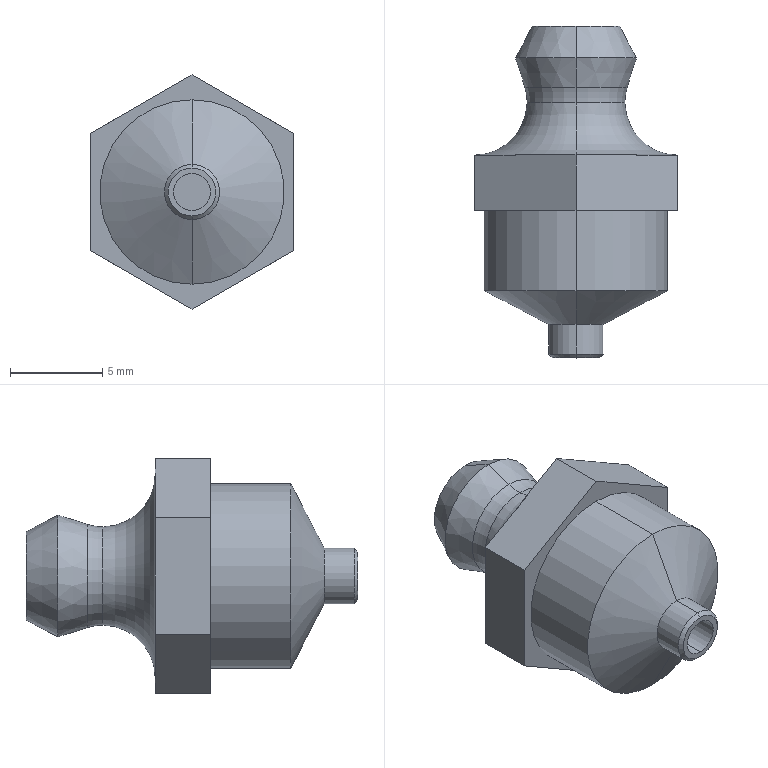Part | SolidWorks | features Boss 1, Chamfer 1, Revolution 1 | 1 solid | 37 faces | box 11 x 18 x 12.702 mm | volume 898.201 mm3 | plane 17 | cone 8 | cylinder 8 | torus 4 | commonest cylinder face diameters 2 x4 3 x2 10 x2
STEP:
#1=CARTESIAN_POINT('',(0.,14.676,2.8));
#2=VERTEX_POINT('',#1);
#3=CARTESIAN_POINT('',(0.,13.829,2.671));
#4=VERTEX_POINT('',#3);
#5=CARTESIAN_POINT('',(0.,13.829,5.5));
#6=DIRECTION('',(-1.,0.,0.));
#7=DIRECTION('',(0.,0.,1.));
#8=AXIS2_PLACEMENT_3D('',#5,#6,#7);
#9=CIRCLE('',#8,2.829);
#10=EDGE_CURVE('',#2,#4,#9,.T.);
#11=ORIENTED_EDGE('',*,*,#10,.T.);
#12=CARTESIAN_POINT('',(0.,13.829,-2.671));
#13=VERTEX_POINT('',#12);
#14=CARTESIAN_POINT('',(0.,13.829,0.));
#15=DIRECTION('',(0.,1.,0.));
#16=DIRECTION('',(0.,0.,1.));
#17=AXIS2_PLACEMENT_3D('',#14,#15,#16);
#18=CIRCLE('',#17,2.671);
#19=EDGE_CURVE('',#4,#13,#18,.T.);
#20=ORIENTED_EDGE('',*,*,#19,.T.);
#21=CARTESIAN_POINT('',(0.,14.676,-2.8));
#22=VERTEX_POINT('',#21);
#23=CARTESIAN_POINT('',(0.,13.829,-5.5));
#24=DIRECTION('',(1.,0.,0.));
#25=DIRECTION('',(0.,0.,-1.));
#26=AXIS2_PLACEMENT_3D('',#23,#24,#25);
#27=CIRCLE('',#26,2.829);
#28=EDGE_CURVE('',#22,#13,#27,.T.);
#29=ORIENTED_EDGE('',*,*,#28,.F.);
#30=CARTESIAN_POINT('',(0.,14.676,0.));
#31=DIRECTION('',(0.,1.,0.));
#32=DIRECTION('',(0.,0.,1.));
#33=AXIS2_PLACEMENT_3D('',#30,#31,#32);
#34=CIRCLE('',#33,2.8);
#35=EDGE_CURVE('',#2,#22,#34,.T.);
#36=ORIENTED_EDGE('',*,*,#35,.F.);
#37=EDGE_LOOP('',(#11,#20,#29,#36));
#38=FACE_OUTER_BOUND('',#37,.T.);
#39=CARTESIAN_POINT('',(0.,13.829,0.));
#40=DIRECTION('',(0.,1.,0.));
#41=DIRECTION('',(0.,0.,1.));
#42=AXIS2_PLACEMENT_3D('',#39,#40,#41);
#43=TOROIDAL_SURFACE('',#42,5.5,2.829);
#44=ADVANCED_FACE('',(#38),#43,.F.);
#45=ORIENTED_EDGE('',*,*,#28,.T.);
#46=CARTESIAN_POINT('',(0.,13.829,0.));
#47=DIRECTION('',(0.,1.,0.));
#48=DIRECTION('',(0.,0.,1.));
#49=AXIS2_PLACEMENT_3D('',#46,#47,#48);
#50=CIRCLE('',#49,2.671);
#51=EDGE_CURVE('',#13,#4,#50,.T.);
#52=ORIENTED_EDGE('',*,*,#51,.T.);
#53=ORIENTED_EDGE('',*,*,#10,.F.);
#54=CARTESIAN_POINT('',(0.,14.676,0.));
#55=DIRECTION('',(0.,1.,0.));
#56=DIRECTION('',(0.,0.,1.));
#57=AXIS2_PLACEMENT_3D('',#54,#55,#56);
#58=CIRCLE('',#57,2.8);
#59=EDGE_CURVE('',#22,#2,#58,.T.);
#60=ORIENTED_EDGE('',*,*,#59,.F.);
#61=EDGE_LOOP('',(#45,#52,#53,#60));
#62=FACE_OUTER_BOUND('',#61,.T.);
#63=CARTESIAN_POINT('',(0.,13.829,0.));
#64=DIRECTION('',(0.,1.,0.));
#65=DIRECTION('',(0.,0.,1.));
#66=AXIS2_PLACEMENT_3D('',#63,#64,#65);
#67=TOROIDAL_SURFACE('',#66,5.5,2.829);
#68=ADVANCED_FACE('',(#62),#67,.F.);
#69=CARTESIAN_POINT('',(0.,0.,-1.3));
#70=VERTEX_POINT('',#69);
#71=CARTESIAN_POINT('',(0.,0.,1.3));
#72=VERTEX_POINT('',#71);
#73=CARTESIAN_POINT('',(0.,0.,0.));
#74=DIRECTION('',(0.,-1.,0.));
#75=DIRECTION('',(0.,0.,-1.));
#76=AXIS2_PLACEMENT_3D('',#73,#74,#75);
#77=CIRCLE('',#76,1.3);
#78=EDGE_CURVE('',#70,#72,#77,.T.);
#79=ORIENTED_EDGE('',*,*,#78,.F.);
#80=CARTESIAN_POINT('',(0.,0.2,-1.5));
#81=VERTEX_POINT('',#80);
#82=CARTESIAN_POINT('',(0.,0.2,-1.5));
#83=DIRECTION('',(0.,0.7071,-0.7071));
#84=VECTOR('',#83,1000.);
#85=LINE('',#82,#84);
#86=EDGE_CURVE('',#70,#81,#85,.T.);
#87=ORIENTED_EDGE('',*,*,#86,.T.);
#88=CARTESIAN_POINT('',(0.,0.2,1.5));
#89=VERTEX_POINT('',#88);
#90=CARTESIAN_POINT('',(0.,0.2,0.));
#91=DIRECTION('',(0.,1.,0.));
#92=DIRECTION('',(0.,0.,-1.));
#93=AXIS2_PLACEMENT_3D('',#90,#91,#92);
#94=CIRCLE('',#93,1.5);
#95=EDGE_CURVE('',#89,#81,#94,.T.);
#96=ORIENTED_EDGE('',*,*,#95,.F.);
#97=CARTESIAN_POINT('',(0.,0.2,1.5));
#98=DIRECTION('',(0.,0.7071,0.7071));
#99=VECTOR('',#98,1000.);
#100=LINE('',#97,#99);
#101=EDGE_CURVE('',#72,#89,#100,.T.);
#102=ORIENTED_EDGE('',*,*,#101,.F.);
#103=EDGE_LOOP('',(#79,#87,#96,#102));
#104=FACE_OUTER_BOUND('',#103,.T.);
#105=CARTESIAN_POINT('',(0.,0.2,0.));
#106=DIRECTION('',(0.,1.,0.));
#107=DIRECTION('',(0.,0.,1.));
#108=AXIS2_PLACEMENT_3D('',#105,#106,#107);
#109=CONICAL_SURFACE('',#108,1.5,0.7854);
#110=ADVANCED_FACE('',(#104),#109,.T.);
#111=ORIENTED_EDGE('',*,*,#51,.F.);
#112=CARTESIAN_POINT('',(0.,11.,-5.5));
#113=VERTEX_POINT('',#112);
#114=CARTESIAN_POINT('',(0.,13.829,-5.5));
#115=DIRECTION('',(1.,0.,0.));
#116=DIRECTION('',(0.,0.,-1.));
#117=AXIS2_PLACEMENT_3D('',#114,#115,#116);
#118=CIRCLE('',#117,2.829);
#119=EDGE_CURVE('',#13,#113,#118,.T.);
#120=ORIENTED_EDGE('',*,*,#119,.T.);
#121=CARTESIAN_POINT('',(-2.75,11.,-4.763));
#122=VERTEX_POINT('',#121);
#123=CARTESIAN_POINT('',(0.,11.,0.));
#124=DIRECTION('',(0.,1.,0.));
#125=DIRECTION('',(0.,0.,1.));
#126=AXIS2_PLACEMENT_3D('',#123,#124,#125);
#127=CIRCLE('',#126,5.5);
#128=EDGE_CURVE('',#113,#122,#127,.T.);
#129=ORIENTED_EDGE('',*,*,#128,.T.);
#130=CARTESIAN_POINT('',(-5.5,11.,0.));
#131=VERTEX_POINT('',#130);
#132=CARTESIAN_POINT('',(0.,11.,0.));
#133=DIRECTION('',(0.,1.,0.));
#134=DIRECTION('',(0.,0.,1.));
#135=AXIS2_PLACEMENT_3D('',#132,#133,#134);
#136=CIRCLE('',#135,5.5);
#137=EDGE_CURVE('',#122,#131,#136,.T.);
#138=ORIENTED_EDGE('',*,*,#137,.T.);
#139=CARTESIAN_POINT('',(-2.75,11.,4.763));
#140=VERTEX_POINT('',#139);
#141=CARTESIAN_POINT('',(0.,11.,0.));
#142=DIRECTION('',(0.,1.,0.));
#143=DIRECTION('',(0.,0.,1.));
#144=AXIS2_PLACEMENT_3D('',#141,#142,#143);
#145=CIRCLE('',#144,5.5);
#146=EDGE_CURVE('',#131,#140,#145,.T.);
#147=ORIENTED_EDGE('',*,*,#146,.T.);
#148=CARTESIAN_POINT('',(0.,11.,5.5));
#149=VERTEX_POINT('',#148);
#150=CARTESIAN_POINT('',(0.,11.,0.));
#151=DIRECTION('',(0.,1.,0.));
#152=DIRECTION('',(0.,0.,1.));
#153=AXIS2_PLACEMENT_3D('',#150,#151,#152);
#154=CIRCLE('',#153,5.5);
#155=EDGE_CURVE('',#140,#149,#154,.T.);
#156=ORIENTED_EDGE('',*,*,#155,.T.);
#157=CARTESIAN_POINT('',(0.,13.829,5.5));
#158=DIRECTION('',(-1.,0.,0.));
#159=DIRECTION('',(0.,0.,1.));
#160=AXIS2_PLACEMENT_3D('',#157,#158,#159);
#161=CIRCLE('',#160,2.829);
#162=EDGE_CURVE('',#4,#149,#161,.T.);
#163=ORIENTED_EDGE('',*,*,#162,.F.);
#164=EDGE_LOOP('',(#111,#120,#129,#138,#147,#156,#163));
#165=FACE_OUTER_BOUND('',#164,.T.);
#166=CARTESIAN_POINT('',(0.,13.829,0.));
#167=DIRECTION('',(0.,1.,0.));
#168=DIRECTION('',(0.,0.,1.));
#169=AXIS2_PLACEMENT_3D('',#166,#167,#168);
#170=TOROIDAL_SURFACE('',#169,5.5,2.829);
#171=ADVANCED_FACE('',(#165),#170,.F.);
#172=ORIENTED_EDGE('',*,*,#35,.T.);
#173=CARTESIAN_POINT('',(0.,16.271,-3.3));
#174=VERTEX_POINT('',#173);
#175=CARTESIAN_POINT('',(0.,16.271,-3.3));
#176=DIRECTION('',(0.,0.9542,-0.299));
#177=VECTOR('',#176,1000.);
#178=LINE('',#175,#177);
#179=EDGE_CURVE('',#22,#174,#178,.T.);
#180=ORIENTED_EDGE('',*,*,#179,.T.);
#181=CARTESIAN_POINT('',(0.,16.271,3.3));
#182=VERTEX_POINT('',#181);
#183=CARTESIAN_POINT('',(0.,16.271,0.));
#184=DIRECTION('',(0.,1.,0.));
#185=DIRECTION('',(0.,0.,1.));
#186=AXIS2_PLACEMENT_3D('',#183,#184,#185);
#187=CIRCLE('',#186,3.3);
#188=EDGE_CURVE('',#182,#174,#187,.T.);
#189=ORIENTED_EDGE('',*,*,#188,.F.);
#190=CARTESIAN_POINT('',(0.,16.271,3.3));
#191=DIRECTION('',(0.,0.9542,0.299));
#192=VECTOR('',#191,1000.);
#193=LINE('',#190,#192);
#194=EDGE_CURVE('',#2,#182,#193,.T.);
#195=ORIENTED_EDGE('',*,*,#194,.F.);
#196=EDGE_LOOP('',(#172,#180,#189,#195));
#197=FACE_OUTER_BOUND('',#196,.T.);
#198=CARTESIAN_POINT('',(0.,16.271,0.));
#199=DIRECTION('',(0.,1.,0.));
#200=DIRECTION('',(0.,0.,1.));
#201=AXIS2_PLACEMENT_3D('',#198,#199,#200);
#202=CONICAL_SURFACE('',#201,3.3,0.3037);
#203=ADVANCED_FACE('',(#197),#202,.T.);
#204=CARTESIAN_POINT('',(0.,18.,2.4));
#205=VERTEX_POINT('',#204);
#206=CARTESIAN_POINT('',(0.,18.,-2.4));
#207=VERTEX_POINT('',#206);
#208=CARTESIAN_POINT('',(0.,18.,0.));
#209=DIRECTION('',(0.,1.,0.));
#210=DIRECTION('',(0.,0.,1.));
#211=AXIS2_PLACEMENT_3D('',#208,#209,#210);
#212=CIRCLE('',#211,2.4);
#213=EDGE_CURVE('',#205,#207,#212,.T.);
#214=ORIENTED_EDGE('',*,*,#213,.F.);
#215=CARTESIAN_POINT('',(0.,18.,2.4));
#216=DIRECTION('',(0.,-0.887,0.4617));
#217=VECTOR('',#216,1000.);
#218=LINE('',#215,#217);
#219=EDGE_CURVE('',#205,#182,#218,.T.);
#220=ORIENTED_EDGE('',*,*,#219,.T.);
#221=ORIENTED_EDGE('',*,*,#188,.T.);
#222=CARTESIAN_POINT('',(0.,18.,-2.4));
#223=DIRECTION('',(0.,-0.887,-0.4617));
#224=VECTOR('',#223,1000.);
#225=LINE('',#222,#224);
#226=EDGE_CURVE('',#207,#174,#225,.T.);
#227=ORIENTED_EDGE('',*,*,#226,.F.);
#228=EDGE_LOOP('',(#214,#220,#221,#227));
#229=FACE_OUTER_BOUND('',#228,.T.);
#230=CARTESIAN_POINT('',(0.,18.,0.));
#231=DIRECTION('',(0.,-1.,0.));
#232=DIRECTION('',(0.,0.,-1.));
#233=AXIS2_PLACEMENT_3D('',#230,#231,#232);
#234=CONICAL_SURFACE('',#233,2.4,0.48);
#235=ADVANCED_FACE('',(#229),#234,.T.);
#236=CARTESIAN_POINT('',(0.,11.,-1.));
#237=VERTEX_POINT('',#236);
#238=CARTESIAN_POINT('',(0.,11.,1.));
#239=VERTEX_POINT('',#238);
#240=CARTESIAN_POINT('',(0.,11.,0.));
#241=DIRECTION('',(0.,1.,0.));
#242=DIRECTION('',(0.,0.,1.));
#243=AXIS2_PLACEMENT_3D('',#240,#241,#242);
#244=CIRCLE('',#243,1.);
#245=EDGE_CURVE('',#237,#239,#244,.T.);
#246=ORIENTED_EDGE('',*,*,#245,.F.);
#247=CARTESIAN_POINT('',(0.,18.,-1.));
#248=VERTEX_POINT('',#247);
#249=CARTESIAN_POINT('',(0.,0.,-1.));
#250=DIRECTION('',(0.,1.,0.));
#251=VECTOR('',#250,1000.);
#252=LINE('',#249,#251);
#253=EDGE_CURVE('',#237,#248,#252,.T.);
#254=ORIENTED_EDGE('',*,*,#253,.T.);
#255=CARTESIAN_POINT('',(0.,18.,1.));
#256=VERTEX_POINT('',#255);
#257=CARTESIAN_POINT('',(0.,18.,0.));
#258=DIRECTION('',(0.,1.,0.));
#259=DIRECTION('',(0.,0.,1.));
#260=AXIS2_PLACEMENT_3D('',#257,#258,#259);
#261=CIRCLE('',#260,1.);
#262=EDGE_CURVE('',#248,#256,#261,.T.);
#263=ORIENTED_EDGE('',*,*,#262,.T.);
#264=CARTESIAN_POINT('',(0.,0.,1.));
#265=DIRECTION('',(0.,1.,0.));
#266=VECTOR('',#265,1000.);
#267=LINE('',#264,#266);
#268=EDGE_CURVE('',#239,#256,#267,.T.);
#269=ORIENTED_EDGE('',*,*,#268,.F.);
#270=EDGE_LOOP('',(#246,#254,#263,#269));
#271=FACE_OUTER_BOUND('',#270,.T.);
#272=CARTESIAN_POINT('',(0.,0.,0.));
#273=DIRECTION('',(0.,1.,0.));
#274=DIRECTION('',(0.,0.,1.));
#275=AXIS2_PLACEMENT_3D('',#272,#273,#274);
#276=CYLINDRICAL_SURFACE('',#275,1.);
#277=ADVANCED_FACE('',(#271),#276,.F.);
#278=ORIENTED_EDGE('',*,*,#95,.T.);
#279=CARTESIAN_POINT('',(0.,1.822,-1.5));
#280=VERTEX_POINT('',#279);
#281=CARTESIAN_POINT('',(0.,0.,-1.5));
#282=DIRECTION('',(0.,1.,0.));
#283=VECTOR('',#282,1000.);
#284=LINE('',#281,#283);
#285=EDGE_CURVE('',#81,#280,#284,.T.);
#286=ORIENTED_EDGE('',*,*,#285,.T.);
#287=CARTESIAN_POINT('',(0.,1.822,1.5));
#288=VERTEX_POINT('',#287);
#289=CARTESIAN_POINT('',(0.,1.822,0.));
#290=DIRECTION('',(0.,1.,0.));
#291=DIRECTION('',(0.,0.,1.));
#292=AXIS2_PLACEMENT_3D('',#289,#290,#291);
#293=CIRCLE('',#292,1.5);
#294=EDGE_CURVE('',#288,#280,#293,.T.);
#295=ORIENTED_EDGE('',*,*,#294,.F.);
#296=CARTESIAN_POINT('',(0.,0.,1.5));
#297=DIRECTION('',(0.,1.,0.));
#298=VECTOR('',#297,1000.);
#299=LINE('',#296,#298);
#300=EDGE_CURVE('',#89,#288,#299,.T.);
#301=ORIENTED_EDGE('',*,*,#300,.F.);
#302=EDGE_LOOP('',(#278,#286,#295,#301));
#303=FACE_OUTER_BOUND('',#302,.T.);
#304=CARTESIAN_POINT('',(0.,0.,0.));
#305=DIRECTION('',(0.,1.,0.));
#306=DIRECTION('',(0.,0.,1.));
#307=AXIS2_PLACEMENT_3D('',#304,#305,#306);
#308=CYLINDRICAL_SURFACE('',#307,1.5);
#309=ADVANCED_FACE('',(#303),#308,.T.);
#310=ORIENTED_EDGE('',*,*,#294,.T.);
#311=CARTESIAN_POINT('',(0.,3.644,-5.));
#312=VERTEX_POINT('',#311);
#313=CARTESIAN_POINT('',(0.,3.644,-5.));
#314=DIRECTION('',(0.,0.4617,-0.887));
#315=VECTOR('',#314,1000.);
#316=LINE('',#313,#315);
#317=EDGE_CURVE('',#280,#312,#316,.T.);
#318=ORIENTED_EDGE('',*,*,#317,.T.);
#319=CARTESIAN_POINT('',(0.,3.644,5.));
#320=VERTEX_POINT('',#319);
#321=CARTESIAN_POINT('',(0.,3.644,0.));
#322=DIRECTION('',(0.,1.,0.));
#323=DIRECTION('',(0.,0.,1.));
#324=AXIS2_PLACEMENT_3D('',#321,#322,#323);
#325=CIRCLE('',#324,5.);
#326=EDGE_CURVE('',#320,#312,#325,.T.);
#327=ORIENTED_EDGE('',*,*,#326,.F.);
#328=CARTESIAN_POINT('',(0.,3.644,5.));
#329=DIRECTION('',(0.,0.4617,0.887));
#330=VECTOR('',#329,1000.);
#331=LINE('',#328,#330);
#332=EDGE_CURVE('',#288,#320,#331,.T.);
#333=ORIENTED_EDGE('',*,*,#332,.F.);
#334=EDGE_LOOP('',(#310,#318,#327,#333));
#335=FACE_OUTER_BOUND('',#334,.T.);
#336=CARTESIAN_POINT('',(0.,3.644,0.));
#337=DIRECTION('',(0.,1.,0.));
#338=DIRECTION('',(0.,0.,1.));
#339=AXIS2_PLACEMENT_3D('',#336,#337,#338);
#340=CONICAL_SURFACE('',#339,5.,1.091);
#341=ADVANCED_FACE('',(#335),#340,.T.);
#342=ORIENTED_EDGE('',*,*,#326,.T.);
#343=CARTESIAN_POINT('',(0.,8.,-5.));
#344=VERTEX_POINT('',#343);
#345=CARTESIAN_POINT('',(0.,0.,-5.));
#346=DIRECTION('',(0.,1.,0.));
#347=VECTOR('',#346,1000.);
#348=LINE('',#345,#347);
#349=EDGE_CURVE('',#312,#344,#348,.T.);
#350=ORIENTED_EDGE('',*,*,#349,.T.);
#351=CARTESIAN_POINT('',(0.,8.,5.));
#352=VERTEX_POINT('',#351);
#353=CARTESIAN_POINT('',(0.,8.,0.));
#354=DIRECTION('',(0.,1.,0.));
#355=DIRECTION('',(0.,0.,1.));
#356=AXIS2_PLACEMENT_3D('',#353,#354,#355);
#357=CIRCLE('',#356,5.);
#358=EDGE_CURVE('',#352,#344,#357,.T.);
#359=ORIENTED_EDGE('',*,*,#358,.F.);
#360=CARTESIAN_POINT('',(0.,0.,5.));
#361=DIRECTION('',(0.,1.,0.));
#362=VECTOR('',#361,1000.);
#363=LINE('',#360,#362);
#364=EDGE_CURVE('',#320,#352,#363,.T.);
#365=ORIENTED_EDGE('',*,*,#364,.F.);
#366=EDGE_LOOP('',(#342,#350,#359,#365));
#367=FACE_OUTER_BOUND('',#366,.T.);
#368=CARTESIAN_POINT('',(0.,0.,0.));
#369=DIRECTION('',(0.,1.,0.));
#370=DIRECTION('',(0.,0.,1.));
#371=AXIS2_PLACEMENT_3D('',#368,#369,#370);
#372=CYLINDRICAL_SURFACE('',#371,5.);
#373=ADVANCED_FACE('',(#367),#372,.T.);
#374=CARTESIAN_POINT('',(0.,0.,-1.));
#375=VERTEX_POINT('',#374);
#376=CARTESIAN_POINT('',(0.,0.,1.));
#377=VERTEX_POINT('',#376);
#378=CARTESIAN_POINT('',(0.,0.,0.));
#379=DIRECTION('',(0.,1.,0.));
#380=DIRECTION('',(0.,0.,1.));
#381=AXIS2_PLACEMENT_3D('',#378,#379,#380);
#382=CIRCLE('',#381,1.);
#383=EDGE_CURVE('',#375,#377,#382,.T.);
#384=ORIENTED_EDGE('',*,*,#383,.F.);
#385=CARTESIAN_POINT('',(0.,8.,-1.));
#386=VERTEX_POINT('',#385);
#387=CARTESIAN_POINT('',(0.,0.,-1.));
#388=DIRECTION('',(0.,1.,0.));
#389=VECTOR('',#388,1000.);
#390=LINE('',#387,#389);
#391=EDGE_CURVE('',#375,#386,#390,.T.);
#392=ORIENTED_EDGE('',*,*,#391,.T.);
#393=CARTESIAN_POINT('',(0.,8.,1.));
#394=VERTEX_POINT('',#393);
#395=CARTESIAN_POINT('',(0.,8.,0.));
#396=DIRECTION('',(0.,1.,0.));
#397=DIRECTION('',(0.,0.,1.));
#398=AXIS2_PLACEMENT_3D('',#395,#396,#397);
#399=CIRCLE('',#398,1.);
#400=EDGE_CURVE('',#386,#394,#399,.T.);
#401=ORIENTED_EDGE('',*,*,#400,.T.);
#402=CARTESIAN_POINT('',(0.,0.,1.));
#403=DIRECTION('',(0.,1.,0.));
#404=VECTOR('',#403,1000.);
#405=LINE('',#402,#404);
#406=EDGE_CURVE('',#377,#394,#405,.T.);
#407=ORIENTED_EDGE('',*,*,#406,.F.);
#408=EDGE_LOOP('',(#384,#392,#401,#407));
#409=FACE_OUTER_BOUND('',#408,.T.);
#410=CARTESIAN_POINT('',(0.,0.,0.));
#411=DIRECTION('',(0.,1.,0.));
#412=DIRECTION('',(0.,0.,1.));
#413=AXIS2_PLACEMENT_3D('',#410,#411,#412);
#414=CYLINDRICAL_SURFACE('',#413,1.);
#415=ADVANCED_FACE('',(#409),#414,.F.);
#416=ORIENTED_EDGE('',*,*,#391,.F.);
#417=CARTESIAN_POINT('',(0.,0.,0.));
#418=DIRECTION('',(0.,1.,0.));
#419=DIRECTION('',(0.,0.,1.));
#420=AXIS2_PLACEMENT_3D('',#417,#418,#419);
#421=CIRCLE('',#420,1.);
#422=EDGE_CURVE('',#377,#375,#421,.T.);
#423=ORIENTED_EDGE('',*,*,#422,.F.);
#424=ORIENTED_EDGE('',*,*,#406,.T.);
#425=CARTESIAN_POINT('',(0.,8.,0.));
#426=DIRECTION('',(0.,1.,0.));
#427=DIRECTION('',(0.,0.,1.));
#428=AXIS2_PLACEMENT_3D('',#425,#426,#427);
#429=CIRCLE('',#428,1.);
#430=EDGE_CURVE('',#394,#386,#429,.T.);
#431=ORIENTED_EDGE('',*,*,#430,.T.);
#432=EDGE_LOOP('',(#416,#423,#424,#431));
#433=FACE_OUTER_BOUND('',#432,.T.);
#434=CARTESIAN_POINT('',(0.,0.,0.));
#435=DIRECTION('',(0.,1.,0.));
#436=DIRECTION('',(0.,0.,1.));
#437=AXIS2_PLACEMENT_3D('',#434,#435,#436);
#438=CYLINDRICAL_SURFACE('',#437,1.);
#439=ADVANCED_FACE('',(#433),#438,.F.);
#440=ORIENTED_EDGE('',*,*,#358,.T.);
#441=CARTESIAN_POINT('',(0.,8.,0.));
#442=DIRECTION('',(0.,1.,0.));
#443=DIRECTION('',(0.,0.,1.));
#444=AXIS2_PLACEMENT_3D('',#441,#442,#443);
#445=CIRCLE('',#444,5.);
#446=EDGE_CURVE('',#344,#352,#445,.T.);
#447=ORIENTED_EDGE('',*,*,#446,.T.);
#448=EDGE_LOOP('',(#440,#447));
#449=FACE_BOUND('',#448,.T.);
#450=CARTESIAN_POINT('',(5.5,8.,3.175));
#451=VERTEX_POINT('',#450);
#452=CARTESIAN_POINT('',(0.,8.,6.351));
#453=VERTEX_POINT('',#452);
#454=CARTESIAN_POINT('',(5.5,8.,3.175));
#455=DIRECTION('',(-0.866,0.,0.5));
#456=VECTOR('',#455,1000.);
#457=LINE('',#454,#456);
#458=EDGE_CURVE('',#451,#453,#457,.T.);
#459=ORIENTED_EDGE('',*,*,#458,.T.);
#460=CARTESIAN_POINT('',(-5.5,8.,3.175));
#461=VERTEX_POINT('',#460);
#462=CARTESIAN_POINT('',(0.,8.,6.351));
#463=DIRECTION('',(-0.866,0.,-0.5));
#464=VECTOR('',#463,1000.);
#465=LINE('',#462,#464);
#466=EDGE_CURVE('',#453,#461,#465,.T.);
#467=ORIENTED_EDGE('',*,*,#466,.T.);
#468=CARTESIAN_POINT('',(-5.5,8.,-3.175));
#469=VERTEX_POINT('',#468);
#470=CARTESIAN_POINT('',(-5.5,8.,3.175));
#471=DIRECTION('',(0.,0.,-1.));
#472=VECTOR('',#471,1000.);
#473=LINE('',#470,#472);
#474=EDGE_CURVE('',#461,#469,#473,.T.);
#475=ORIENTED_EDGE('',*,*,#474,.T.);
#476=CARTESIAN_POINT('',(0.,8.,-6.351));
#477=VERTEX_POINT('',#476);
#478=CARTESIAN_POINT('',(-5.5,8.,-3.175));
#479=DIRECTION('',(0.866,0.,-0.5));
#480=VECTOR('',#479,1000.);
#481=LINE('',#478,#480);
#482=EDGE_CURVE('',#469,#477,#481,.T.);
#483=ORIENTED_EDGE('',*,*,#482,.T.);
#484=CARTESIAN_POINT('',(5.5,8.,-3.175));
#485=VERTEX_POINT('',#484);
#486=CARTESIAN_POINT('',(0.,8.,-6.351));
#487=DIRECTION('',(0.866,0.,0.5));
#488=VECTOR('',#487,1000.);
#489=LINE('',#486,#488);
#490=EDGE_CURVE('',#477,#485,#489,.T.);
#491=ORIENTED_EDGE('',*,*,#490,.T.);
#492=CARTESIAN_POINT('',(5.5,8.,-3.175));
#493=DIRECTION('',(0.,0.,1.));
#494=VECTOR('',#493,1000.);
#495=LINE('',#492,#494);
#496=EDGE_CURVE('',#485,#451,#495,.T.);
#497=ORIENTED_EDGE('',*,*,#496,.T.);
#498=EDGE_LOOP('',(#459,#467,#475,#483,#491,#497));
#499=FACE_OUTER_BOUND('',#498,.T.);
#500=CARTESIAN_POINT('',(-5.,8.,0.));
#501=DIRECTION('',(0.,-1.,0.));
#502=DIRECTION('',(0.,0.,-1.));
#503=AXIS2_PLACEMENT_3D('',#500,#501,#502);
#504=PLANE('',#503);
#505=ADVANCED_FACE('',(#449,#499),#504,.T.);
#506=ORIENTED_EDGE('',*,*,#349,.F.);
#507=CARTESIAN_POINT('',(0.,3.644,0.));
#508=DIRECTION('',(0.,1.,0.));
#509=DIRECTION('',(0.,0.,1.));
#510=AXIS2_PLACEMENT_3D('',#507,#508,#509);
#511=CIRCLE('',#510,5.);
#512=EDGE_CURVE('',#312,#320,#511,.T.);
#513=ORIENTED_EDGE('',*,*,#512,.T.);
#514=ORIENTED_EDGE('',*,*,#364,.T.);
#515=ORIENTED_EDGE('',*,*,#446,.F.);
#516=EDGE_LOOP('',(#506,#513,#514,#515));
#517=FACE_OUTER_BOUND('',#516,.T.);
#518=CARTESIAN_POINT('',(0.,0.,0.));
#519=DIRECTION('',(0.,1.,0.));
#520=DIRECTION('',(0.,0.,1.));
#521=AXIS2_PLACEMENT_3D('',#518,#519,#520);
#522=CYLINDRICAL_SURFACE('',#521,5.);
#523=ADVANCED_FACE('',(#517),#522,.T.);
#524=ORIENTED_EDGE('',*,*,#317,.F.);
#525=CARTESIAN_POINT('',(0.,1.822,0.));
#526=DIRECTION('',(0.,1.,0.));
#527=DIRECTION('',(0.,0.,1.));
#528=AXIS2_PLACEMENT_3D('',#525,#526,#527);
#529=CIRCLE('',#528,1.5);
#530=EDGE_CURVE('',#280,#288,#529,.T.);
#531=ORIENTED_EDGE('',*,*,#530,.T.);
#532=ORIENTED_EDGE('',*,*,#332,.T.);
#533=ORIENTED_EDGE('',*,*,#512,.F.);
#534=EDGE_LOOP('',(#524,#531,#532,#533));
#535=FACE_OUTER_BOUND('',#534,.T.);
#536=CARTESIAN_POINT('',(0.,3.644,0.));
#537=DIRECTION('',(0.,1.,0.));
#538=DIRECTION('',(0.,0.,1.));
#539=AXIS2_PLACEMENT_3D('',#536,#537,#538);
#540=CONICAL_SURFACE('',#539,5.,1.091);
#541=ADVANCED_FACE('',(#535),#540,.T.);
#542=ORIENTED_EDGE('',*,*,#285,.F.);
#543=CARTESIAN_POINT('',(0.,0.2,0.));
#544=DIRECTION('',(0.,1.,0.));
#545=DIRECTION('',(0.,0.,-1.));
#546=AXIS2_PLACEMENT_3D('',#543,#544,#545);
#547=CIRCLE('',#546,1.5);
#548=EDGE_CURVE('',#81,#89,#547,.T.);
#549=ORIENTED_EDGE('',*,*,#548,.T.);
#550=ORIENTED_EDGE('',*,*,#300,.T.);
#551=ORIENTED_EDGE('',*,*,#530,.F.);
#552=EDGE_LOOP('',(#542,#549,#550,#551));
#553=FACE_OUTER_BOUND('',#552,.T.);
#554=CARTESIAN_POINT('',(0.,0.,0.));
#555=DIRECTION('',(0.,1.,0.));
#556=DIRECTION('',(0.,0.,1.));
#557=AXIS2_PLACEMENT_3D('',#554,#555,#556);
#558=CYLINDRICAL_SURFACE('',#557,1.5);
#559=ADVANCED_FACE('',(#553),#558,.T.);
#560=CARTESIAN_POINT('',(0.,0.,0.));
#561=DIRECTION('',(0.,-1.,0.));
#562=DIRECTION('',(0.,0.,-1.));
#563=AXIS2_PLACEMENT_3D('',#560,#561,#562);
#564=CIRCLE('',#563,1.3);
#565=EDGE_CURVE('',#72,#70,#564,.T.);
#566=ORIENTED_EDGE('',*,*,#565,.T.);
#567=ORIENTED_EDGE('',*,*,#78,.T.);
#568=EDGE_LOOP('',(#566,#567));
#569=FACE_OUTER_BOUND('',#568,.T.);
#570=ORIENTED_EDGE('',*,*,#422,.T.);
#571=ORIENTED_EDGE('',*,*,#383,.T.);
#572=EDGE_LOOP('',(#570,#571));
#573=FACE_BOUND('',#572,.T.);
#574=CARTESIAN_POINT('',(-1.,0.,0.));
#575=DIRECTION('',(0.,-1.,0.));
#576=DIRECTION('',(0.,0.,-1.));
#577=AXIS2_PLACEMENT_3D('',#574,#575,#576);
#578=PLANE('',#577);
#579=ADVANCED_FACE('',(#569,#573),#578,.T.);
#580=CARTESIAN_POINT('',(2.75,11.,4.763));
#581=VERTEX_POINT('',#580);
#582=CARTESIAN_POINT('',(0.,11.,6.351));
#583=VERTEX_POINT('',#582);
#584=CARTESIAN_POINT('',(5.5,11.,3.175));
#585=DIRECTION('',(-0.866,0.,0.5));
#586=VECTOR('',#585,1000.);
#587=LINE('',#584,#586);
#588=EDGE_CURVE('',#581,#583,#587,.T.);
#589=ORIENTED_EDGE('',*,*,#588,.F.);
#590=CARTESIAN_POINT('',(0.,11.,0.));
#591=DIRECTION('',(0.,1.,0.));
#592=DIRECTION('',(0.,0.,1.));
#593=AXIS2_PLACEMENT_3D('',#590,#591,#592);
#594=CIRCLE('',#593,5.5);
#595=EDGE_CURVE('',#149,#581,#594,.T.);
#596=ORIENTED_EDGE('',*,*,#595,.F.);
#597=ORIENTED_EDGE('',*,*,#155,.F.);
#598=CARTESIAN_POINT('',(0.,11.,6.351));
#599=DIRECTION('',(-0.866,0.,-0.5));
#600=VECTOR('',#599,1000.);
#601=LINE('',#598,#600);
#602=EDGE_CURVE('',#583,#140,#601,.T.);
#603=ORIENTED_EDGE('',*,*,#602,.F.);
#604=EDGE_LOOP('',(#589,#596,#597,#603));
#605=FACE_OUTER_BOUND('',#604,.T.);
#606=CARTESIAN_POINT('',(0.,11.,6.351));
#607=DIRECTION('',(0.,1.,0.));
#608=DIRECTION('',(0.,0.,1.));
#609=AXIS2_PLACEMENT_3D('',#606,#607,#608);
#610=PLANE('',#609);
#611=ADVANCED_FACE('',(#605),#610,.T.);
#612=CARTESIAN_POINT('',(-5.5,11.,-3.175));
#613=VERTEX_POINT('',#612);
#614=CARTESIAN_POINT('',(-5.5,11.,-3.175));
#615=DIRECTION('',(0.,-1.,0.));
#616=VECTOR('',#615,1000.);
#617=LINE('',#614,#616);
#618=EDGE_CURVE('',#613,#469,#617,.T.);
#619=ORIENTED_EDGE('',*,*,#618,.T.);
#620=ORIENTED_EDGE('',*,*,#474,.F.);
#621=CARTESIAN_POINT('',(-5.5,11.,3.175));
#622=VERTEX_POINT('',#621);
#623=CARTESIAN_POINT('',(-5.5,11.,3.175));
#624=DIRECTION('',(0.,-1.,0.));
#625=VECTOR('',#624,1000.);
#626=LINE('',#623,#625);
#627=EDGE_CURVE('',#622,#461,#626,.T.);
#628=ORIENTED_EDGE('',*,*,#627,.F.);
#629=CARTESIAN_POINT('',(-5.5,11.,3.175));
#630=DIRECTION('',(0.,0.,-1.));
#631=VECTOR('',#630,1000.);
#632=LINE('',#629,#631);
#633=EDGE_CURVE('',#622,#131,#632,.T.);
#634=ORIENTED_EDGE('',*,*,#633,.T.);
#635=CARTESIAN_POINT('',(-5.5,11.,3.175));
#636=DIRECTION('',(0.,0.,-1.));
#637=VECTOR('',#636,1000.);
#638=LINE('',#635,#637);
#639=EDGE_CURVE('',#131,#613,#638,.T.);
#640=ORIENTED_EDGE('',*,*,#639,.T.);
#641=EDGE_LOOP('',(#619,#620,#628,#634,#640));
#642=FACE_OUTER_BOUND('',#641,.T.);
#643=CARTESIAN_POINT('',(-5.5,11.,3.175));
#644=DIRECTION('',(-1.,0.,0.));
#645=DIRECTION('',(0.,0.,1.));
#646=AXIS2_PLACEMENT_3D('',#643,#644,#645);
#647=PLANE('',#646);
#648=ADVANCED_FACE('',(#642),#647,.T.);
#649=CARTESIAN_POINT('',(0.,11.,-6.351));
#650=VERTEX_POINT('',#649);
#651=CARTESIAN_POINT('',(0.,11.,-6.351));
#652=DIRECTION('',(0.,-1.,0.));
#653=VECTOR('',#652,1000.);
#654=LINE('',#651,#653);
#655=EDGE_CURVE('',#650,#477,#654,.T.);
#656=ORIENTED_EDGE('',*,*,#655,.T.);
#657=ORIENTED_EDGE('',*,*,#482,.F.);
#658=ORIENTED_EDGE('',*,*,#618,.F.);
#659=CARTESIAN_POINT('',(-5.5,11.,-3.175));
#660=DIRECTION('',(0.866,0.,-0.5));
#661=VECTOR('',#660,1000.);
#662=LINE('',#659,#661);
#663=EDGE_CURVE('',#613,#122,#662,.T.);
#664=ORIENTED_EDGE('',*,*,#663,.T.);
#665=CARTESIAN_POINT('',(-5.5,11.,-3.175));
#666=DIRECTION('',(0.866,0.,-0.5));
#667=VECTOR('',#666,1000.);
#668=LINE('',#665,#667);
#669=EDGE_CURVE('',#122,#650,#668,.T.);
#670=ORIENTED_EDGE('',*,*,#669,.T.);
#671=EDGE_LOOP('',(#656,#657,#658,#664,#670));
#672=FACE_OUTER_BOUND('',#671,.T.);
#673=CARTESIAN_POINT('',(-5.5,11.,-3.175));
#674=DIRECTION('',(-0.5,0.,-0.866));
#675=DIRECTION('',(-0.866,0.,0.5));
#676=AXIS2_PLACEMENT_3D('',#673,#674,#675);
#677=PLANE('',#676);
#678=ADVANCED_FACE('',(#672),#677,.T.);
#679=CARTESIAN_POINT('',(5.5,11.,-3.175));
#680=VERTEX_POINT('',#679);
#681=CARTESIAN_POINT('',(5.5,11.,-3.175));
#682=DIRECTION('',(0.,-1.,0.));
#683=VECTOR('',#682,1000.);
#684=LINE('',#681,#683);
#685=EDGE_CURVE('',#680,#485,#684,.T.);
#686=ORIENTED_EDGE('',*,*,#685,.T.);
#687=ORIENTED_EDGE('',*,*,#490,.F.);
#688=ORIENTED_EDGE('',*,*,#655,.F.);
#689=CARTESIAN_POINT('',(2.75,11.,-4.763));
#690=VERTEX_POINT('',#689);
#691=CARTESIAN_POINT('',(0.,11.,-6.351));
#692=DIRECTION('',(0.866,0.,0.5));
#693=VECTOR('',#692,1000.);
#694=LINE('',#691,#693);
#695=EDGE_CURVE('',#650,#690,#694,.T.);
#696=ORIENTED_EDGE('',*,*,#695,.T.);
#697=CARTESIAN_POINT('',(0.,11.,-6.351));
#698=DIRECTION('',(0.866,0.,0.5));
#699=VECTOR('',#698,1000.);
#700=LINE('',#697,#699);
#701=EDGE_CURVE('',#690,#680,#700,.T.);
#702=ORIENTED_EDGE('',*,*,#701,.T.);
#703=EDGE_LOOP('',(#686,#687,#688,#696,#702));
#704=FACE_OUTER_BOUND('',#703,.T.);
#705=CARTESIAN_POINT('',(0.,11.,-6.351));
#706=DIRECTION('',(0.5,0.,-0.866));
#707=DIRECTION('',(-0.866,0.,-0.5));
#708=AXIS2_PLACEMENT_3D('',#705,#706,#707);
#709=PLANE('',#708);
#710=ADVANCED_FACE('',(#704),#709,.T.);
#711=CARTESIAN_POINT('',(5.5,11.,3.175));
#712=VERTEX_POINT('',#711);
#713=CARTESIAN_POINT('',(5.5,11.,3.175));
#714=DIRECTION('',(0.,-1.,0.));
#715=VECTOR('',#714,1000.);
#716=LINE('',#713,#715);
#717=EDGE_CURVE('',#712,#451,#716,.T.);
#718=ORIENTED_EDGE('',*,*,#717,.T.);
#719=ORIENTED_EDGE('',*,*,#496,.F.);
#720=ORIENTED_EDGE('',*,*,#685,.F.);
#721=CARTESIAN_POINT('',(5.5,11.,0.));
#722=VERTEX_POINT('',#721);
#723=CARTESIAN_POINT('',(5.5,11.,-3.175));
#724=DIRECTION('',(0.,0.,1.));
#725=VECTOR('',#724,1000.);
#726=LINE('',#723,#725);
#727=EDGE_CURVE('',#680,#722,#726,.T.);
#728=ORIENTED_EDGE('',*,*,#727,.T.);
#729=CARTESIAN_POINT('',(5.5,11.,-3.175));
#730=DIRECTION('',(0.,0.,1.));
#731=VECTOR('',#730,1000.);
#732=LINE('',#729,#731);
#733=EDGE_CURVE('',#722,#712,#732,.T.);
#734=ORIENTED_EDGE('',*,*,#733,.T.);
#735=EDGE_LOOP('',(#718,#719,#720,#728,#734));
#736=FACE_OUTER_BOUND('',#735,.T.);
#737=CARTESIAN_POINT('',(5.5,11.,-3.175));
#738=DIRECTION('',(1.,0.,0.));
#739=DIRECTION('',(0.,0.,-1.));
#740=AXIS2_PLACEMENT_3D('',#737,#738,#739);
#741=PLANE('',#740);
#742=ADVANCED_FACE('',(#736),#741,.T.);
#743=CARTESIAN_POINT('',(0.,11.,6.351));
#744=DIRECTION('',(0.,-1.,0.));
#745=VECTOR('',#744,1000.);
#746=LINE('',#743,#745);
#747=EDGE_CURVE('',#583,#453,#746,.T.);
#748=ORIENTED_EDGE('',*,*,#747,.T.);
#749=ORIENTED_EDGE('',*,*,#458,.F.);
#750=ORIENTED_EDGE('',*,*,#717,.F.);
#751=CARTESIAN_POINT('',(5.5,11.,3.175));
#752=DIRECTION('',(-0.866,0.,0.5));
#753=VECTOR('',#752,1000.);
#754=LINE('',#751,#753);
#755=EDGE_CURVE('',#712,#581,#754,.T.);
#756=ORIENTED_EDGE('',*,*,#755,.T.);
#757=ORIENTED_EDGE('',*,*,#588,.T.);
#758=EDGE_LOOP('',(#748,#749,#750,#756,#757));
#759=FACE_OUTER_BOUND('',#758,.T.);
#760=CARTESIAN_POINT('',(5.5,11.,3.175));
#761=DIRECTION('',(0.5,0.,0.866));
#762=DIRECTION('',(0.866,0.,-0.5));
#763=AXIS2_PLACEMENT_3D('',#760,#761,#762);
#764=PLANE('',#763);
#765=ADVANCED_FACE('',(#759),#764,.T.);
#766=ORIENTED_EDGE('',*,*,#466,.F.);
#767=ORIENTED_EDGE('',*,*,#747,.F.);
#768=ORIENTED_EDGE('',*,*,#602,.T.);
#769=CARTESIAN_POINT('',(0.,11.,6.351));
#770=DIRECTION('',(-0.866,0.,-0.5));
#771=VECTOR('',#770,1000.);
#772=LINE('',#769,#771);
#773=EDGE_CURVE('',#140,#622,#772,.T.);
#774=ORIENTED_EDGE('',*,*,#773,.T.);
#775=ORIENTED_EDGE('',*,*,#627,.T.);
#776=EDGE_LOOP('',(#766,#767,#768,#774,#775));
#777=FACE_OUTER_BOUND('',#776,.T.);
#778=CARTESIAN_POINT('',(0.,11.,6.351));
#779=DIRECTION('',(-0.5,0.,0.866));
#780=DIRECTION('',(0.866,0.,0.5));
#781=AXIS2_PLACEMENT_3D('',#778,#779,#780);
#782=PLANE('',#781);
#783=ADVANCED_FACE('',(#777),#782,.T.);
#784=ORIENTED_EDGE('',*,*,#733,.F.);
#785=CARTESIAN_POINT('',(0.,11.,0.));
#786=DIRECTION('',(0.,1.,0.));
#787=DIRECTION('',(0.,0.,1.));
#788=AXIS2_PLACEMENT_3D('',#785,#786,#787);
#789=CIRCLE('',#788,5.5);
#790=EDGE_CURVE('',#581,#722,#789,.T.);
#791=ORIENTED_EDGE('',*,*,#790,.F.);
#792=ORIENTED_EDGE('',*,*,#755,.F.);
#793=EDGE_LOOP('',(#784,#791,#792));
#794=FACE_OUTER_BOUND('',#793,.T.);
#795=CARTESIAN_POINT('',(0.,11.,6.351));
#796=DIRECTION('',(0.,1.,0.));
#797=DIRECTION('',(0.,0.,1.));
#798=AXIS2_PLACEMENT_3D('',#795,#796,#797);
#799=PLANE('',#798);
#800=ADVANCED_FACE('',(#794),#799,.T.);
#801=ORIENTED_EDGE('',*,*,#701,.F.);
#802=CARTESIAN_POINT('',(0.,11.,0.));
#803=DIRECTION('',(0.,1.,0.));
#804=DIRECTION('',(0.,0.,1.));
#805=AXIS2_PLACEMENT_3D('',#802,#803,#804);
#806=CIRCLE('',#805,5.5);
#807=EDGE_CURVE('',#722,#690,#806,.T.);
#808=ORIENTED_EDGE('',*,*,#807,.F.);
#809=ORIENTED_EDGE('',*,*,#727,.F.);
#810=EDGE_LOOP('',(#801,#808,#809));
#811=FACE_OUTER_BOUND('',#810,.T.);
#812=CARTESIAN_POINT('',(0.,11.,6.351));
#813=DIRECTION('',(0.,1.,0.));
#814=DIRECTION('',(0.,0.,1.));
#815=AXIS2_PLACEMENT_3D('',#812,#813,#814);
#816=PLANE('',#815);
#817=ADVANCED_FACE('',(#811),#816,.T.);
#818=ORIENTED_EDGE('',*,*,#669,.F.);
#819=ORIENTED_EDGE('',*,*,#128,.F.);
#820=CARTESIAN_POINT('',(0.,11.,0.));
#821=DIRECTION('',(0.,1.,0.));
#822=DIRECTION('',(0.,0.,1.));
#823=AXIS2_PLACEMENT_3D('',#820,#821,#822);
#824=CIRCLE('',#823,5.5);
#825=EDGE_CURVE('',#690,#113,#824,.T.);
#826=ORIENTED_EDGE('',*,*,#825,.F.);
#827=ORIENTED_EDGE('',*,*,#695,.F.);
#828=EDGE_LOOP('',(#818,#819,#826,#827));
#829=FACE_OUTER_BOUND('',#828,.T.);
#830=CARTESIAN_POINT('',(0.,11.,6.351));
#831=DIRECTION('',(0.,1.,0.));
#832=DIRECTION('',(0.,0.,1.));
#833=AXIS2_PLACEMENT_3D('',#830,#831,#832);
#834=PLANE('',#833);
#835=ADVANCED_FACE('',(#829),#834,.T.);
#836=ORIENTED_EDGE('',*,*,#639,.F.);
#837=ORIENTED_EDGE('',*,*,#137,.F.);
#838=ORIENTED_EDGE('',*,*,#663,.F.);
#839=EDGE_LOOP('',(#836,#837,#838));
#840=FACE_OUTER_BOUND('',#839,.T.);
#841=CARTESIAN_POINT('',(0.,11.,6.351));
#842=DIRECTION('',(0.,1.,0.));
#843=DIRECTION('',(0.,0.,1.));
#844=AXIS2_PLACEMENT_3D('',#841,#842,#843);
#845=PLANE('',#844);
#846=ADVANCED_FACE('',(#840),#845,.T.);
#847=ORIENTED_EDGE('',*,*,#773,.F.);
#848=ORIENTED_EDGE('',*,*,#146,.F.);
#849=ORIENTED_EDGE('',*,*,#633,.F.);
#850=EDGE_LOOP('',(#847,#848,#849));
#851=FACE_OUTER_BOUND('',#850,.T.);
#852=CARTESIAN_POINT('',(0.,11.,6.351));
#853=DIRECTION('',(0.,1.,0.));
#854=DIRECTION('',(0.,0.,1.));
#855=AXIS2_PLACEMENT_3D('',#852,#853,#854);
#856=PLANE('',#855);
#857=ADVANCED_FACE('',(#851),#856,.T.);
#858=CARTESIAN_POINT('',(0.,18.,0.));
#859=DIRECTION('',(0.,1.,0.));
#860=DIRECTION('',(0.,0.,1.));
#861=AXIS2_PLACEMENT_3D('',#858,#859,#860);
#862=CIRCLE('',#861,2.4);
#863=EDGE_CURVE('',#207,#205,#862,.T.);
#864=ORIENTED_EDGE('',*,*,#863,.T.);
#865=ORIENTED_EDGE('',*,*,#213,.T.);
#866=EDGE_LOOP('',(#864,#865));
#867=FACE_OUTER_BOUND('',#866,.T.);
#868=CARTESIAN_POINT('',(0.,18.,0.));
#869=DIRECTION('',(0.,1.,0.));
#870=DIRECTION('',(0.,0.,1.));
#871=AXIS2_PLACEMENT_3D('',#868,#869,#870);
#872=CIRCLE('',#871,1.);
#873=EDGE_CURVE('',#256,#248,#872,.T.);
#874=ORIENTED_EDGE('',*,*,#873,.F.);
#875=ORIENTED_EDGE('',*,*,#262,.F.);
#876=EDGE_LOOP('',(#874,#875));
#877=FACE_BOUND('',#876,.T.);
#878=CARTESIAN_POINT('',(-1.,18.,0.));
#879=DIRECTION('',(0.,1.,0.));
#880=DIRECTION('',(0.,0.,1.));
#881=AXIS2_PLACEMENT_3D('',#878,#879,#880);
#882=PLANE('',#881);
#883=ADVANCED_FACE('',(#867,#877),#882,.T.);
#884=ORIENTED_EDGE('',*,*,#253,.F.);
#885=CARTESIAN_POINT('',(0.,11.,0.));
#886=DIRECTION('',(0.,1.,0.));
#887=DIRECTION('',(0.,0.,1.));
#888=AXIS2_PLACEMENT_3D('',#885,#886,#887);
#889=CIRCLE('',#888,1.);
#890=EDGE_CURVE('',#239,#237,#889,.T.);
#891=ORIENTED_EDGE('',*,*,#890,.F.);
#892=ORIENTED_EDGE('',*,*,#268,.T.);
#893=ORIENTED_EDGE('',*,*,#873,.T.);
#894=EDGE_LOOP('',(#884,#891,#892,#893));
#895=FACE_OUTER_BOUND('',#894,.T.);
#896=CARTESIAN_POINT('',(0.,0.,0.));
#897=DIRECTION('',(0.,1.,0.));
#898=DIRECTION('',(0.,0.,1.));
#899=AXIS2_PLACEMENT_3D('',#896,#897,#898);
#900=CYLINDRICAL_SURFACE('',#899,1.);
#901=ADVANCED_FACE('',(#895),#900,.F.);
#902=ORIENTED_EDGE('',*,*,#219,.F.);
#903=ORIENTED_EDGE('',*,*,#863,.F.);
#904=ORIENTED_EDGE('',*,*,#226,.T.);
#905=CARTESIAN_POINT('',(0.,16.271,0.));
#906=DIRECTION('',(0.,1.,0.));
#907=DIRECTION('',(0.,0.,1.));
#908=AXIS2_PLACEMENT_3D('',#905,#906,#907);
#909=CIRCLE('',#908,3.3);
#910=EDGE_CURVE('',#174,#182,#909,.T.);
#911=ORIENTED_EDGE('',*,*,#910,.T.);
#912=EDGE_LOOP('',(#902,#903,#904,#911));
#913=FACE_OUTER_BOUND('',#912,.T.);
#914=CARTESIAN_POINT('',(0.,18.,0.));
#915=DIRECTION('',(0.,-1.,0.));
#916=DIRECTION('',(0.,0.,-1.));
#917=AXIS2_PLACEMENT_3D('',#914,#915,#916);
#918=CONICAL_SURFACE('',#917,2.4,0.48);
#919=ADVANCED_FACE('',(#913),#918,.T.);
#920=ORIENTED_EDGE('',*,*,#179,.F.);
#921=ORIENTED_EDGE('',*,*,#59,.T.);
#922=ORIENTED_EDGE('',*,*,#194,.T.);
#923=ORIENTED_EDGE('',*,*,#910,.F.);
#924=EDGE_LOOP('',(#920,#921,#922,#923));
#925=FACE_OUTER_BOUND('',#924,.T.);
#926=CARTESIAN_POINT('',(0.,16.271,0.));
#927=DIRECTION('',(0.,1.,0.));
#928=DIRECTION('',(0.,0.,1.));
#929=AXIS2_PLACEMENT_3D('',#926,#927,#928);
#930=CONICAL_SURFACE('',#929,3.3,0.3037);
#931=ADVANCED_FACE('',(#925),#930,.T.);
#932=ORIENTED_EDGE('',*,*,#19,.F.);
#933=ORIENTED_EDGE('',*,*,#162,.T.);
#934=ORIENTED_EDGE('',*,*,#595,.T.);
#935=ORIENTED_EDGE('',*,*,#790,.T.);
#936=ORIENTED_EDGE('',*,*,#807,.T.);
#937=ORIENTED_EDGE('',*,*,#825,.T.);
#938=ORIENTED_EDGE('',*,*,#119,.F.);
#939=EDGE_LOOP('',(#932,#933,#934,#935,#936,#937,#938));
#940=FACE_OUTER_BOUND('',#939,.T.);
#941=CARTESIAN_POINT('',(0.,13.829,0.));
#942=DIRECTION('',(0.,1.,0.));
#943=DIRECTION('',(0.,0.,1.));
#944=AXIS2_PLACEMENT_3D('',#941,#942,#943);
#945=TOROIDAL_SURFACE('',#944,5.5,2.829);
#946=ADVANCED_FACE('',(#940),#945,.F.);
#947=ORIENTED_EDGE('',*,*,#430,.F.);
#948=ORIENTED_EDGE('',*,*,#400,.F.);
#949=EDGE_LOOP('',(#947,#948));
#950=FACE_OUTER_BOUND('',#949,.T.);
#951=CARTESIAN_POINT('',(0.,8.,6.351));
#952=DIRECTION('',(0.,1.,0.));
#953=DIRECTION('',(0.,0.,1.));
#954=AXIS2_PLACEMENT_3D('',#951,#952,#953);
#955=PLANE('',#954);
#956=ADVANCED_FACE('',(#950),#955,.F.);
#957=ORIENTED_EDGE('',*,*,#890,.T.);
#958=ORIENTED_EDGE('',*,*,#245,.T.);
#959=EDGE_LOOP('',(#957,#958));
#960=FACE_OUTER_BOUND('',#959,.T.);
#961=CARTESIAN_POINT('',(0.,11.,6.351));
#962=DIRECTION('',(0.,1.,0.));
#963=DIRECTION('',(0.,0.,1.));
#964=AXIS2_PLACEMENT_3D('',#961,#962,#963);
#965=PLANE('',#964);
#966=ADVANCED_FACE('',(#960),#965,.T.);
#967=ORIENTED_EDGE('',*,*,#86,.F.);
#968=ORIENTED_EDGE('',*,*,#565,.F.);
#969=ORIENTED_EDGE('',*,*,#101,.T.);
#970=ORIENTED_EDGE('',*,*,#548,.F.);
#971=EDGE_LOOP('',(#967,#968,#969,#970));
#972=FACE_OUTER_BOUND('',#971,.T.);
#973=CARTESIAN_POINT('',(0.,0.2,0.));
#974=DIRECTION('',(0.,1.,0.));
#975=DIRECTION('',(0.,0.,1.));
#976=AXIS2_PLACEMENT_3D('',#973,#974,#975);
#977=CONICAL_SURFACE('',#976,1.5,0.7854);
#978=ADVANCED_FACE('',(#972),#977,.T.);
#979=CLOSED_SHELL('',(#44,#68,#110,#171,#203,#235,#277,#309,#341,#373,#415,#439,#505,#523,#541,#559,#579,#611,#648,#678,#710,#742,#765,#783,#800,#817,#835,#846,#857,#883,#901,#919,#931,#946,#956,#966,#978));
#980=MANIFOLD_SOLID_BREP('',#979);
#981=CARTESIAN_POINT('',(0.,0.,0.));
#982=DIRECTION('',(0.,0.,1.));
#983=DIRECTION('',(1.,0.,0.));
#984=AXIS2_PLACEMENT_3D('',#981,#982,#983);
#985=(LENGTH_UNIT()NAMED_UNIT(*)SI_UNIT(.MILLI.,.METRE.));
#986=UNCERTAINTY_MEASURE_WITH_UNIT(LENGTH_MEASURE(0.00001),#985,'','');
#987=(NAMED_UNIT(*)PLANE_ANGLE_UNIT()SI_UNIT($,.RADIAN.));
#988=(NAMED_UNIT(*)SI_UNIT($,.STERADIAN.)SOLID_ANGLE_UNIT());
#989=(GEOMETRIC_REPRESENTATION_CONTEXT(3)GLOBAL_UNCERTAINTY_ASSIGNED_CONTEXT((#986))GLOBAL_UNIT_ASSIGNED_CONTEXT((#985,#987,#988))REPRESENTATION_CONTEXT('',''));
#990=ADVANCED_BREP_SHAPE_REPRESENTATION('',(#980,#984),#989);